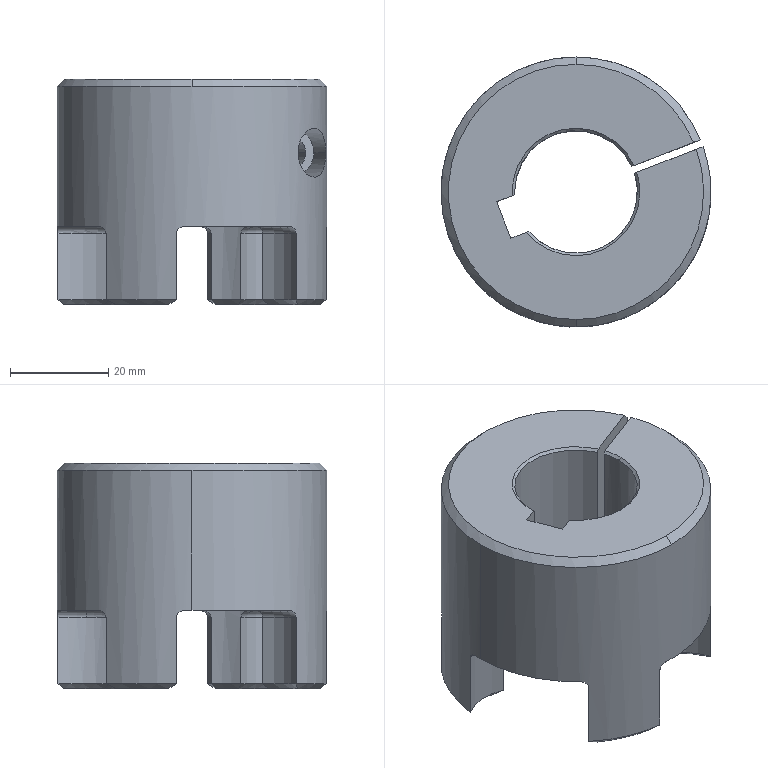Part | NX | features BREP 1 | 1 solid | 76 faces | box 55 x 55 x 46 mm | volume 59296 mm3 | cone 26 | cylinder 24 | plane 17 | torus 9 | commonest cylinder face diameters 22.734 x9 25 x3 35 x3 55 x3 5 x2 6.5 x2